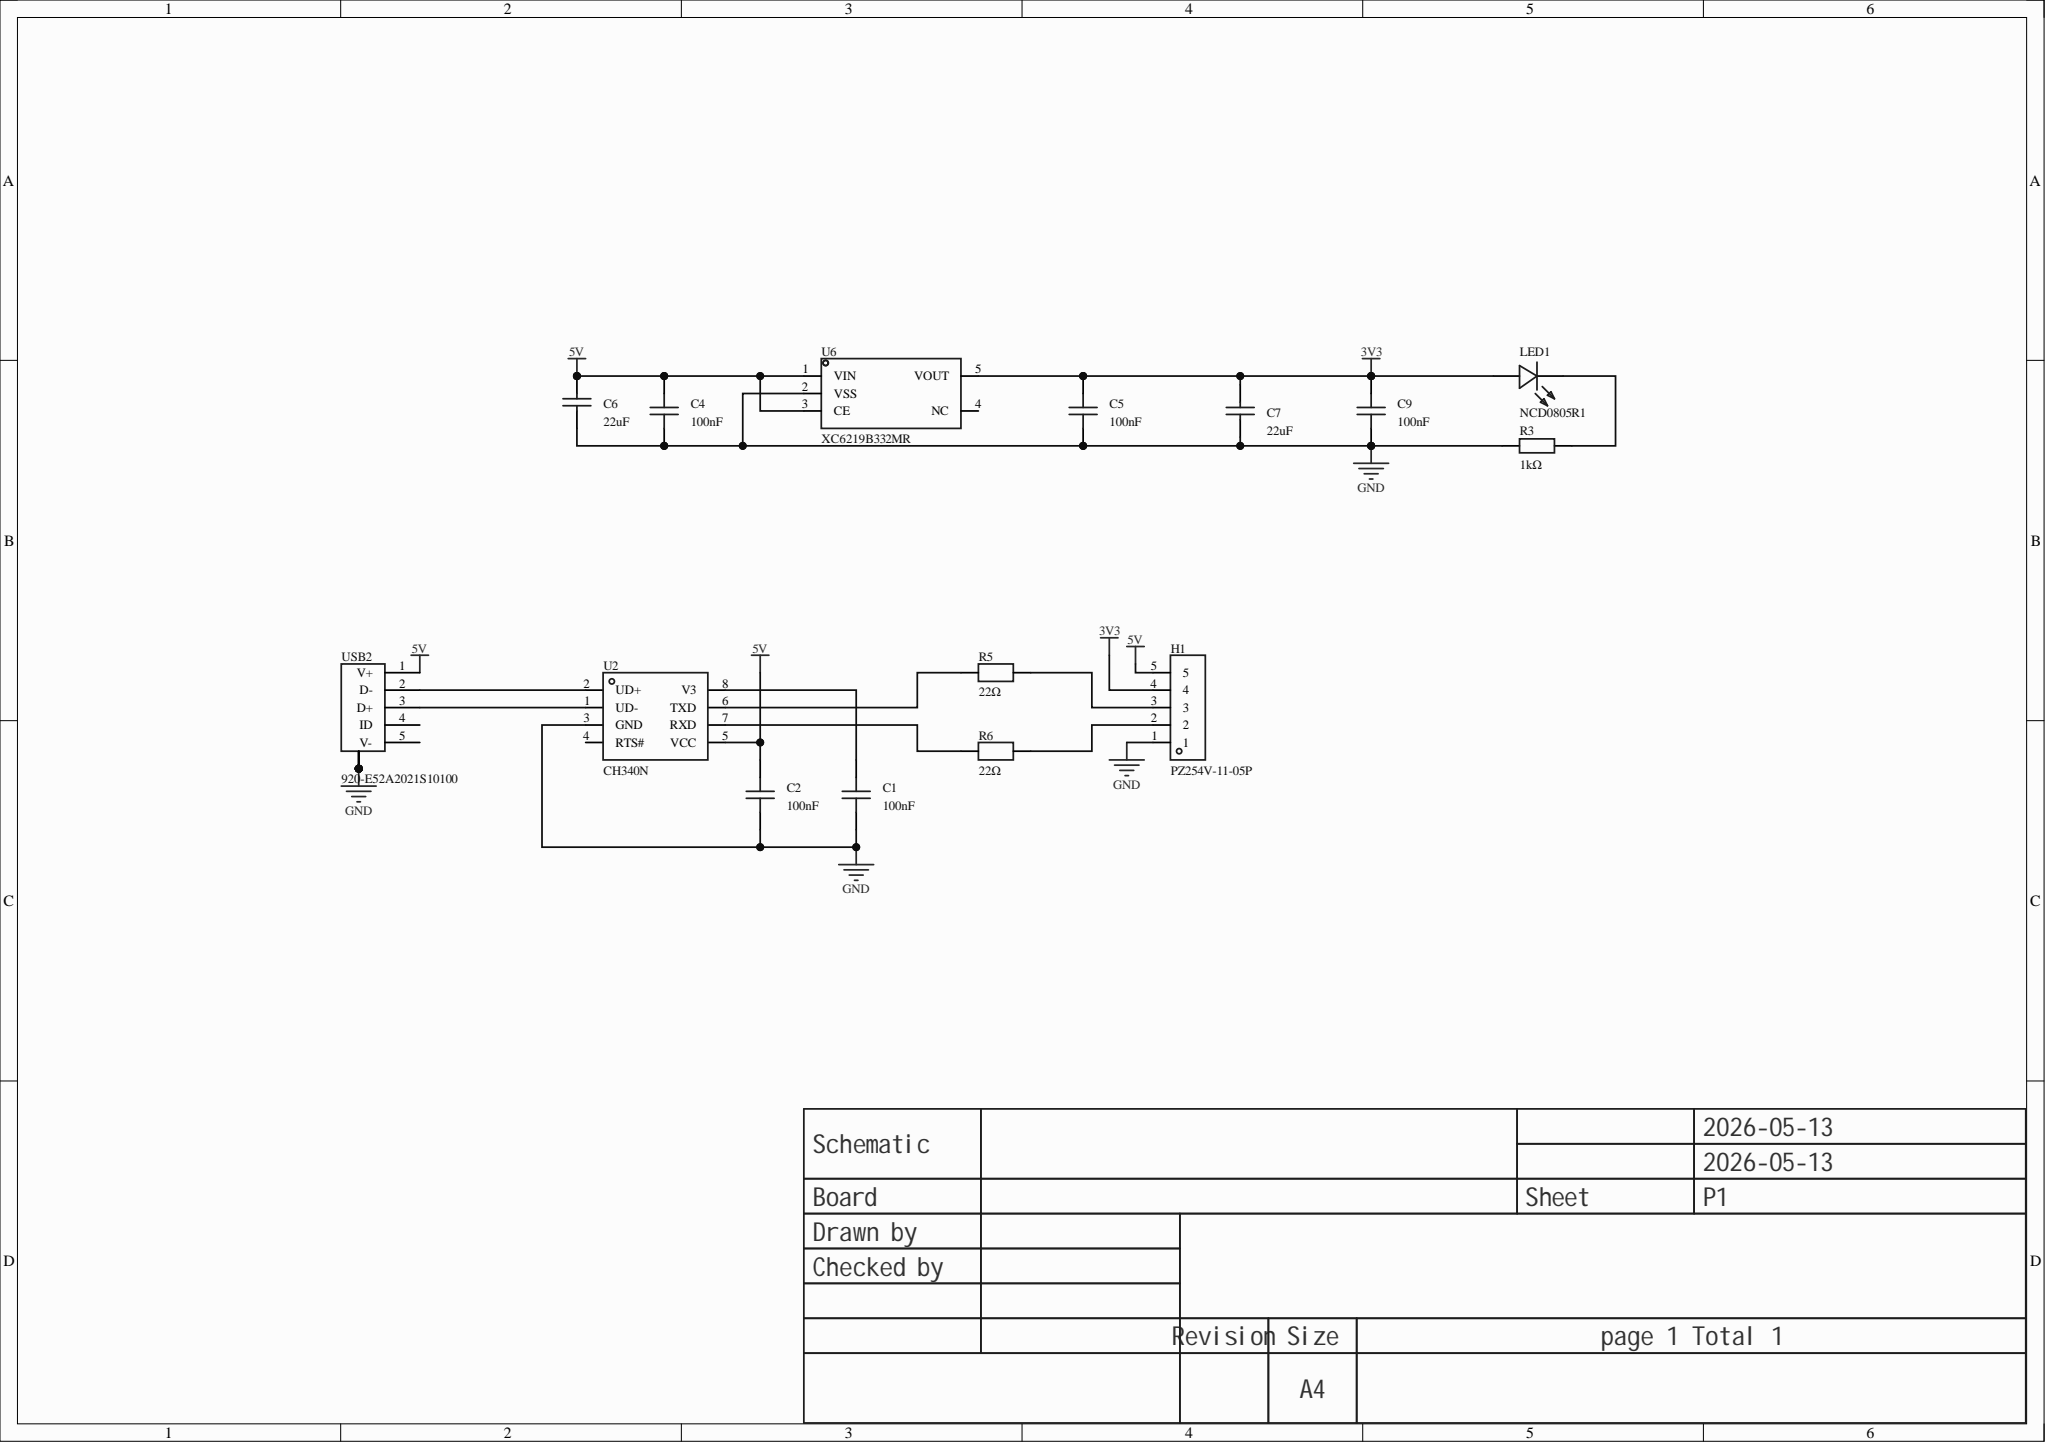Circuit board | Altium Designer | 15 parts | 11 nets
Bill of materials:
Comment,Description,Designator,Footprint,LibRef,Quantity
"100nF","Capacitance:100nF;Tolerance:±10%;Rated voltage:50V;Temperature coefficient:X7R;, Capacitance:100nF;Tolerance:±10%;Rated voltage:50V;Temperature coefficient (material):X7R;","C1, C2, C4, C5, C9","C0603","CC0603KRX7R9BB104, 0603BB104K500NGT","5"
"22uF","Capacitance:22uF;Tolerance:±20%;Rated voltage:6.3V;Temperature coefficient:X5R;","C6, C7","C0805","0805X226M6R3NT","2"
"PZ254V-11-05P","Pin structure:1x5P;Pitch:2.54mm;Row spacing:-;Square/round pin:Square pin;Mounting:Through-hole;Rows:Single row;Total pins:5P;Rated current:3A;Rated voltage:250V;Mating pin length:6mm;Plastic height:2.5mm;Termination pin length:3mm;Contact material:Brass;Contact plating:-;Operating temperature:-40℃~+105℃;Color:Black;","H1","HDR-TH_5P-P2.54-V-M","PZ254V-11-05P","1"
"NCD0805R1","Lamp head type:-;Emitted color:Red;Forward voltage (Vf):1.6V~2.6V;Power:65mW;Forward current:25mA;Wavelength:615nm~630nm;Diode configuration:Single diode;Lens color:-;Color temperature:-;Luminous intensity:195mcd;Viewing angle:130°;Tape packaging:-;Operating temperature:-30℃~+85℃;","LED1","LED0805-RD","NCD0805R1","1"
"1kΩ","Resistor type:Thick film resistor;Resistance:1kΩ;Tolerance:±1%;Power:100mW;Operating voltage:75V;Temperature coefficient:±100ppm/?;","R3","R0603","0603WAF1001T5E","1"
"22Ω","Resistor type:Thick film resistor;Resistance:22Ω;Tolerance:±5%;Power:100mW;Maximum operating voltage:75V;","R5, R6","R0603","SCR0603J22R","2"
"CH340N","Application function:USB to serial;USB protocol version:USB 2.0;Channels:1;Data rate:2Mbps;","U2","SOP-8_L4.9-W3.9-P1.27-LS6.0-BL","CH340N","1"
"XC6219B332MR","Output type:Fixed;Operating voltage:7V;Output voltage:3.3V;Output current:300mA;Power supply rejection ratio (PSRR):40dB@(1kHz);Output polarity:Positive;","U6","SOT-23-5_L3.0-W1.7-P0.95-LS2.8-BR","XC6219B332MR_C347386","1"
"920-E52A2021S10100","Connector type:Micro-B;Protocol standard:USB 2.0;Gender:Female;Mounting:Horizontal mount;Contact count:5P;Port count:1;Rated current - power:1A;Operating temperature:-30℃~+80℃;","USB2","MICRO-USB-SMD_5P-P0.65-H-F_C10418","920-E52A2021S10100","1"
Netlist (Protel format):
[
C1
C0603
100nF



]
[
C2
C0603
100nF



]
[
C4
C0603
100nF



]
[
C5
C0603
100nF



]
[
C6
C0805
22uF



]
[
C7
C0805
22uF



]
[
C9
C0603
100nF



]
[
H1
HDR-TH_5P-P2.54-V-M
PZ254V-11-05P



]
[
LED1
LED0805-RD
NCD0805R1



]
[
R3
R0603
1kΩ



]
[
R5
R0603
22Ω



]
[
R6
R0603
22Ω



]
[
U2
SOP-8_L4.9-W3.9-P1.27-LS6.0-BL
CH340N



]
[
U6
SOT-23-5_L3.0-W1.7-P0.95-LS2.8-BR
XC6219B332MR



]
[
USB2
MICRO-USB-SMD_5P-P0.65-H-F_C10418
920-E52A2021S10100



]
(
NetU2_2
U2-2
USB2-2
)
(
NetU2_1
U2-1
USB2-3
)
(
NetR6_1
R6-1
U2-7
)
(
NetR5_1
R5-1
U2-6
)
(
NetLED1_1
LED1-1
R3-2
)
(
NetH1_3
H1-3
R5-2
)
(
NetH1_2
H1-2
R6-2
)
(
NetC1_2
C1-2
U2-8
)
(
GND
C1-1
C2-1
C4-1
C5-1
C6-1
C7-1
C9-1
H1-1
R3-1
U2-3
U6-2
USB2-SH0
USB2-SH1
USB2-SH2
USB2-SH3
)
(
5V
C2-2
C4-2
C6-2
H1-5
U2-5
U6-1
U6-3
USB2-1
)
(
3V3
C5-2
C7-2
C9-2
H1-4
LED1-2
U6-5
)